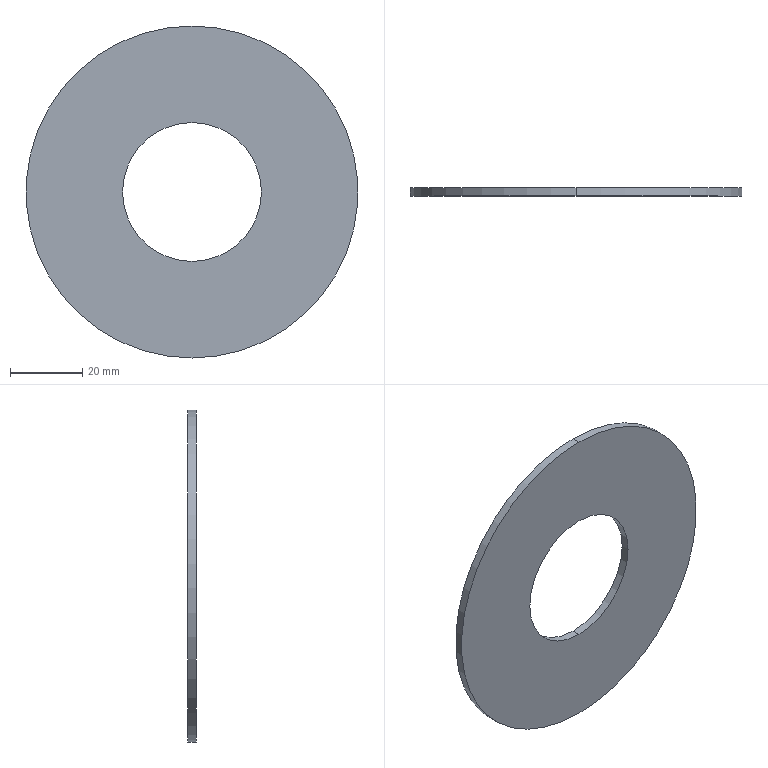Part | SolidWorks | features FlatPattern 1, SMBaseFlange 1, SheetMetal 1 | 1 solid | 6 faces | box 92 x 2.3 x 92 mm | volume 12612 mm3 | cylinder 4 | plane 2 | commonest cylinder face diameters 38.5 x2 92 x2
STEP:
#1=CARTESIAN_POINT('',(0.,-2.3,-19.25));
#2=VERTEX_POINT('',#1);
#3=CARTESIAN_POINT('',(0.,-2.3,19.25));
#4=VERTEX_POINT('',#3);
#5=CARTESIAN_POINT('',(0.,-2.3,0.));
#6=DIRECTION('',(0.,1.,0.));
#7=DIRECTION('',(0.,0.,1.));
#8=AXIS2_PLACEMENT_3D('',#5,#6,#7);
#9=CIRCLE('',#8,19.25);
#10=EDGE_CURVE('',#2,#4,#9,.T.);
#11=ORIENTED_EDGE('',*,*,#10,.F.);
#12=CARTESIAN_POINT('',(0.,0.,-19.25));
#13=VERTEX_POINT('',#12);
#14=CARTESIAN_POINT('',(0.,-2.3,-19.25));
#15=DIRECTION('',(0.,1.,0.));
#16=VECTOR('',#15,1000.);
#17=LINE('',#14,#16);
#18=EDGE_CURVE('',#2,#13,#17,.T.);
#19=ORIENTED_EDGE('',*,*,#18,.T.);
#20=CARTESIAN_POINT('',(0.,0.,19.25));
#21=VERTEX_POINT('',#20);
#22=CARTESIAN_POINT('',(0.,0.,0.));
#23=DIRECTION('',(0.,1.,0.));
#24=DIRECTION('',(0.,0.,1.));
#25=AXIS2_PLACEMENT_3D('',#22,#23,#24);
#26=CIRCLE('',#25,19.25);
#27=EDGE_CURVE('',#13,#21,#26,.T.);
#28=ORIENTED_EDGE('',*,*,#27,.T.);
#29=CARTESIAN_POINT('',(0.,-2.3,19.25));
#30=DIRECTION('',(0.,1.,0.));
#31=VECTOR('',#30,1000.);
#32=LINE('',#29,#31);
#33=EDGE_CURVE('',#4,#21,#32,.T.);
#34=ORIENTED_EDGE('',*,*,#33,.F.);
#35=EDGE_LOOP('',(#11,#19,#28,#34));
#36=FACE_OUTER_BOUND('',#35,.T.);
#37=CARTESIAN_POINT('',(0.,-2.3,0.));
#38=DIRECTION('',(0.,1.,0.));
#39=DIRECTION('',(0.,0.,1.));
#40=AXIS2_PLACEMENT_3D('',#37,#38,#39);
#41=CYLINDRICAL_SURFACE('',#40,19.25);
#42=ADVANCED_FACE('',(#36),#41,.F.);
#43=CARTESIAN_POINT('',(0.,-2.3,46.));
#44=VERTEX_POINT('',#43);
#45=CARTESIAN_POINT('',(0.,-2.3,-46.));
#46=VERTEX_POINT('',#45);
#47=CARTESIAN_POINT('',(0.,-2.3,0.));
#48=DIRECTION('',(0.,1.,0.));
#49=DIRECTION('',(0.,0.,1.));
#50=AXIS2_PLACEMENT_3D('',#47,#48,#49);
#51=CIRCLE('',#50,46.);
#52=EDGE_CURVE('',#44,#46,#51,.T.);
#53=ORIENTED_EDGE('',*,*,#52,.T.);
#54=CARTESIAN_POINT('',(0.,0.,-46.));
#55=VERTEX_POINT('',#54);
#56=CARTESIAN_POINT('',(0.,-2.3,-46.));
#57=DIRECTION('',(0.,1.,0.));
#58=VECTOR('',#57,1000.);
#59=LINE('',#56,#58);
#60=EDGE_CURVE('',#46,#55,#59,.T.);
#61=ORIENTED_EDGE('',*,*,#60,.T.);
#62=CARTESIAN_POINT('',(0.,0.,46.));
#63=VERTEX_POINT('',#62);
#64=CARTESIAN_POINT('',(0.,0.,0.));
#65=DIRECTION('',(0.,1.,0.));
#66=DIRECTION('',(0.,0.,1.));
#67=AXIS2_PLACEMENT_3D('',#64,#65,#66);
#68=CIRCLE('',#67,46.);
#69=EDGE_CURVE('',#63,#55,#68,.T.);
#70=ORIENTED_EDGE('',*,*,#69,.F.);
#71=CARTESIAN_POINT('',(0.,-2.3,46.));
#72=DIRECTION('',(0.,1.,0.));
#73=VECTOR('',#72,1000.);
#74=LINE('',#71,#73);
#75=EDGE_CURVE('',#44,#63,#74,.T.);
#76=ORIENTED_EDGE('',*,*,#75,.F.);
#77=EDGE_LOOP('',(#53,#61,#70,#76));
#78=FACE_OUTER_BOUND('',#77,.T.);
#79=CARTESIAN_POINT('',(0.,-2.3,0.));
#80=DIRECTION('',(0.,1.,0.));
#81=DIRECTION('',(0.,0.,1.));
#82=AXIS2_PLACEMENT_3D('',#79,#80,#81);
#83=CYLINDRICAL_SURFACE('',#82,46.);
#84=ADVANCED_FACE('',(#78),#83,.T.);
#85=ORIENTED_EDGE('',*,*,#60,.F.);
#86=CARTESIAN_POINT('',(0.,-2.3,0.));
#87=DIRECTION('',(0.,1.,0.));
#88=DIRECTION('',(0.,0.,1.));
#89=AXIS2_PLACEMENT_3D('',#86,#87,#88);
#90=CIRCLE('',#89,46.);
#91=EDGE_CURVE('',#46,#44,#90,.T.);
#92=ORIENTED_EDGE('',*,*,#91,.T.);
#93=ORIENTED_EDGE('',*,*,#75,.T.);
#94=CARTESIAN_POINT('',(0.,0.,0.));
#95=DIRECTION('',(0.,1.,0.));
#96=DIRECTION('',(0.,0.,1.));
#97=AXIS2_PLACEMENT_3D('',#94,#95,#96);
#98=CIRCLE('',#97,46.);
#99=EDGE_CURVE('',#55,#63,#98,.T.);
#100=ORIENTED_EDGE('',*,*,#99,.F.);
#101=EDGE_LOOP('',(#85,#92,#93,#100));
#102=FACE_OUTER_BOUND('',#101,.T.);
#103=CARTESIAN_POINT('',(0.,-2.3,0.));
#104=DIRECTION('',(0.,1.,0.));
#105=DIRECTION('',(0.,0.,1.));
#106=AXIS2_PLACEMENT_3D('',#103,#104,#105);
#107=CYLINDRICAL_SURFACE('',#106,46.);
#108=ADVANCED_FACE('',(#102),#107,.T.);
#109=CARTESIAN_POINT('',(0.,-2.3,0.));
#110=DIRECTION('',(0.,1.,0.));
#111=DIRECTION('',(0.,0.,1.));
#112=AXIS2_PLACEMENT_3D('',#109,#110,#111);
#113=CIRCLE('',#112,19.25);
#114=EDGE_CURVE('',#4,#2,#113,.T.);
#115=ORIENTED_EDGE('',*,*,#114,.T.);
#116=ORIENTED_EDGE('',*,*,#10,.T.);
#117=EDGE_LOOP('',(#115,#116));
#118=FACE_BOUND('',#117,.T.);
#119=ORIENTED_EDGE('',*,*,#52,.F.);
#120=ORIENTED_EDGE('',*,*,#91,.F.);
#121=EDGE_LOOP('',(#119,#120));
#122=FACE_OUTER_BOUND('',#121,.T.);
#123=CARTESIAN_POINT('',(0.,-2.3,0.));
#124=DIRECTION('',(0.,1.,0.));
#125=DIRECTION('',(0.,0.,1.));
#126=AXIS2_PLACEMENT_3D('',#123,#124,#125);
#127=PLANE('',#126);
#128=ADVANCED_FACE('',(#118,#122),#127,.F.);
#129=CARTESIAN_POINT('',(0.,0.,0.));
#130=DIRECTION('',(0.,1.,0.));
#131=DIRECTION('',(0.,0.,1.));
#132=AXIS2_PLACEMENT_3D('',#129,#130,#131);
#133=CIRCLE('',#132,19.25);
#134=EDGE_CURVE('',#21,#13,#133,.T.);
#135=ORIENTED_EDGE('',*,*,#134,.F.);
#136=ORIENTED_EDGE('',*,*,#27,.F.);
#137=EDGE_LOOP('',(#135,#136));
#138=FACE_BOUND('',#137,.T.);
#139=ORIENTED_EDGE('',*,*,#69,.T.);
#140=ORIENTED_EDGE('',*,*,#99,.T.);
#141=EDGE_LOOP('',(#139,#140));
#142=FACE_OUTER_BOUND('',#141,.T.);
#143=CARTESIAN_POINT('',(0.,0.,0.));
#144=DIRECTION('',(0.,1.,0.));
#145=DIRECTION('',(0.,0.,1.));
#146=AXIS2_PLACEMENT_3D('',#143,#144,#145);
#147=PLANE('',#146);
#148=ADVANCED_FACE('',(#138,#142),#147,.T.);
#149=ORIENTED_EDGE('',*,*,#18,.F.);
#150=ORIENTED_EDGE('',*,*,#114,.F.);
#151=ORIENTED_EDGE('',*,*,#33,.T.);
#152=ORIENTED_EDGE('',*,*,#134,.T.);
#153=EDGE_LOOP('',(#149,#150,#151,#152));
#154=FACE_OUTER_BOUND('',#153,.T.);
#155=CARTESIAN_POINT('',(0.,-2.3,0.));
#156=DIRECTION('',(0.,1.,0.));
#157=DIRECTION('',(0.,0.,1.));
#158=AXIS2_PLACEMENT_3D('',#155,#156,#157);
#159=CYLINDRICAL_SURFACE('',#158,19.25);
#160=ADVANCED_FACE('',(#154),#159,.F.);
#161=CLOSED_SHELL('',(#42,#84,#108,#128,#148,#160));
#162=MANIFOLD_SOLID_BREP('',#161);
#163=CARTESIAN_POINT('',(0.,0.,0.));
#164=DIRECTION('',(0.,0.,1.));
#165=DIRECTION('',(1.,0.,0.));
#166=AXIS2_PLACEMENT_3D('',#163,#164,#165);
#167=(LENGTH_UNIT()NAMED_UNIT(*)SI_UNIT(.MILLI.,.METRE.));
#168=UNCERTAINTY_MEASURE_WITH_UNIT(LENGTH_MEASURE(0.00001),#167,'','');
#169=(NAMED_UNIT(*)PLANE_ANGLE_UNIT()SI_UNIT($,.RADIAN.));
#170=(NAMED_UNIT(*)SI_UNIT($,.STERADIAN.)SOLID_ANGLE_UNIT());
#171=(GEOMETRIC_REPRESENTATION_CONTEXT(3)GLOBAL_UNCERTAINTY_ASSIGNED_CONTEXT((#168))GLOBAL_UNIT_ASSIGNED_CONTEXT((#167,#169,#170))REPRESENTATION_CONTEXT('',''));
#172=ADVANCED_BREP_SHAPE_REPRESENTATION('',(#162,#166),#171);